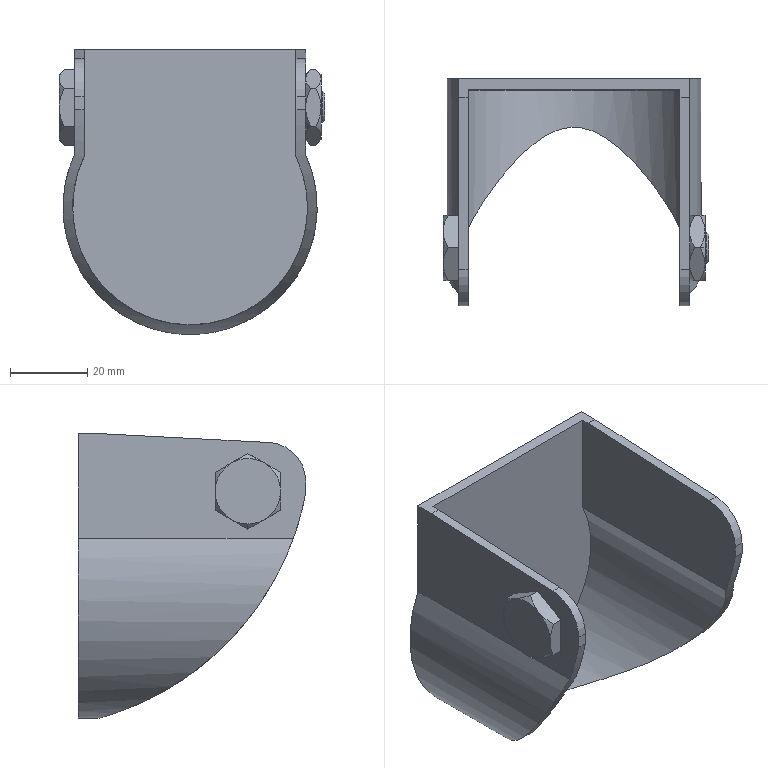Part | SolidWorks | features BaseBody 1 | 1 solid | 55 faces | box 69 x 59 x 74 mm | volume 31525 mm3 | plane 26 | cone 22 | cylinder 7 | commonest cylinder face diameters 8 x2 20 x2 61 x1 66 x1 150 x1